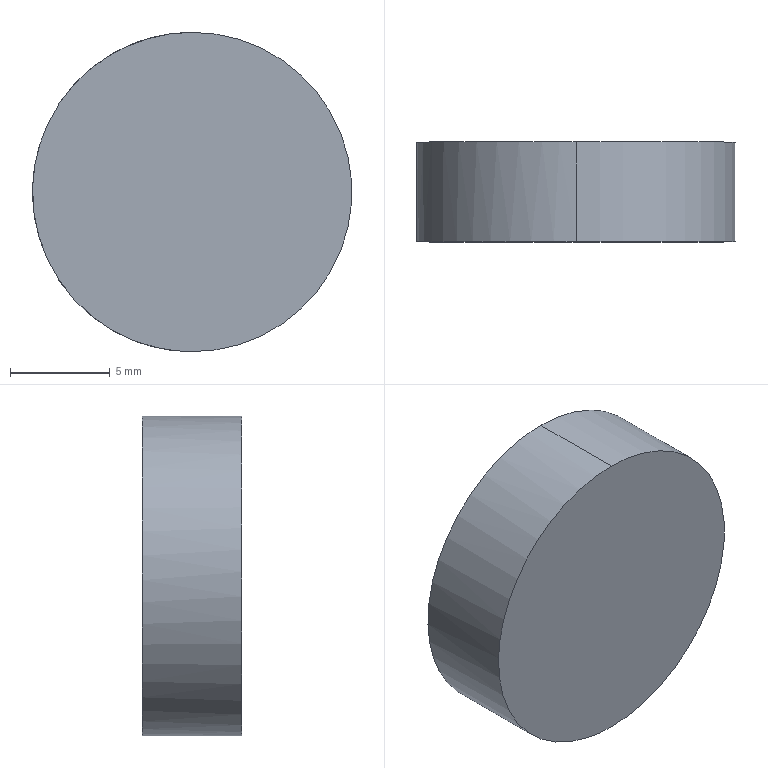Part | STEP file | Positioning_id1206_x_t | 1 solid | 4 faces | box 16 x 5 x 16 mm | volume 1005 mm3 | cylinder 2 | plane 2 | commonest cylinder face diameters 16 x2
STEP:
#1=CARTESIAN_POINT('',(0.,0.,0.));
#2=DIRECTION('',(0.,0.,1.));
#3=DIRECTION('',(1.,0.,0.));
#4=AXIS2_PLACEMENT_3D('',#1,#2,#3);
#5=CARTESIAN_POINT('',(-767.002,214.,185.532));
#6=VERTEX_POINT('',#5);
#7=CARTESIAN_POINT('',(-767.002,219.,185.532));
#8=VERTEX_POINT('',#7);
#9=CARTESIAN_POINT('',(-767.002,219.,185.532));
#10=DIRECTION('',(0.,1.,0.));
#11=VECTOR('',#10,1.);
#12=LINE('',#9,#11);
#13=CARTESIAN_POINT('',(-767.002,219.,193.532));
#14=DIRECTION('',(0.,1.,0.));
#15=DIRECTION('',(0.,0.,-1.));
#16=AXIS2_PLACEMENT_3D('',#13,#14,#15);
#17=CYLINDRICAL_SURFACE('',#16,8.);
#18=CARTESIAN_POINT('',(6.283,0.));
#19=DIRECTION('',(0.,1.));
#20=VECTOR('',#19,1.);
#21=LINE('',#18,#20);
#22=(GEOMETRIC_REPRESENTATION_CONTEXT(2)PARAMETRIC_REPRESENTATION_CONTEXT()REPRESENTATION_CONTEXT('',''));
#23=DEFINITIONAL_REPRESENTATION('',(#21),#22);
#24=PCURVE('',#17,#23);
#25=CARTESIAN_POINT('',(-767.002,219.,193.532));
#26=DIRECTION('',(0.,1.,0.));
#27=DIRECTION('',(0.,0.,-1.));
#28=AXIS2_PLACEMENT_3D('',#25,#26,#27);
#29=CYLINDRICAL_SURFACE('',#28,8.);
#30=CARTESIAN_POINT('',(0.,0.));
#31=DIRECTION('',(0.,1.));
#32=VECTOR('',#31,1.);
#33=LINE('',#30,#32);
#34=(GEOMETRIC_REPRESENTATION_CONTEXT(2)PARAMETRIC_REPRESENTATION_CONTEXT()REPRESENTATION_CONTEXT('',''));
#35=DEFINITIONAL_REPRESENTATION('',(#33),#34);
#36=PCURVE('',#29,#35);
#37=SURFACE_CURVE('',#12,(#24,#36),.PCURVE_S1.);
#38=EDGE_CURVE('',#6,#8,#37,.T.);
#39=ORIENTED_EDGE('',*,*,#38,.T.);
#40=CARTESIAN_POINT('',(-767.002,219.,201.532));
#41=VERTEX_POINT('',#40);
#42=CARTESIAN_POINT('',(-767.002,219.,193.532));
#43=DIRECTION('',(0.,1.,0.));
#44=DIRECTION('',(0.,0.,1.));
#45=AXIS2_PLACEMENT_3D('',#42,#43,#44);
#46=CIRCLE('',#45,8.);
#47=CARTESIAN_POINT('',(3.142,0.));
#48=DIRECTION('',(1.,0.));
#49=VECTOR('',#48,1.);
#50=LINE('',#47,#49);
#51=(GEOMETRIC_REPRESENTATION_CONTEXT(2)PARAMETRIC_REPRESENTATION_CONTEXT()REPRESENTATION_CONTEXT('',''));
#52=DEFINITIONAL_REPRESENTATION('',(#50),#51);
#53=PCURVE('',#17,#52);
#54=CARTESIAN_POINT('',(-767.002,219.,193.532));
#55=DIRECTION('',(0.,1.,0.));
#56=DIRECTION('',(0.,0.,1.));
#57=AXIS2_PLACEMENT_3D('',#54,#55,#56);
#58=PLANE('',#57);
#59=CARTESIAN_POINT('',(0.,0.));
#60=DIRECTION('',(1.,0.));
#61=AXIS2_PLACEMENT_2D('',#59,#60);
#62=CIRCLE('',#61,8.);
#63=(GEOMETRIC_REPRESENTATION_CONTEXT(2)PARAMETRIC_REPRESENTATION_CONTEXT()REPRESENTATION_CONTEXT('',''));
#64=DEFINITIONAL_REPRESENTATION('',(#62),#63);
#65=PCURVE('',#58,#64);
#66=SURFACE_CURVE('',#46,(#53,#65),.PCURVE_S1.);
#67=EDGE_CURVE('',#41,#8,#66,.T.);
#68=ORIENTED_EDGE('',*,*,#67,.F.);
#69=CARTESIAN_POINT('',(-767.002,214.,201.532));
#70=VERTEX_POINT('',#69);
#71=CARTESIAN_POINT('',(-767.002,219.,201.532));
#72=DIRECTION('',(0.,-1.,0.));
#73=VECTOR('',#72,1.);
#74=LINE('',#71,#73);
#75=CARTESIAN_POINT('',(3.142,0.));
#76=DIRECTION('',(0.,-1.));
#77=VECTOR('',#76,1.);
#78=LINE('',#75,#77);
#79=(GEOMETRIC_REPRESENTATION_CONTEXT(2)PARAMETRIC_REPRESENTATION_CONTEXT()REPRESENTATION_CONTEXT('',''));
#80=DEFINITIONAL_REPRESENTATION('',(#78),#79);
#81=PCURVE('',#17,#80);
#82=CARTESIAN_POINT('',(3.142,0.));
#83=DIRECTION('',(0.,-1.));
#84=VECTOR('',#83,1.);
#85=LINE('',#82,#84);
#86=(GEOMETRIC_REPRESENTATION_CONTEXT(2)PARAMETRIC_REPRESENTATION_CONTEXT()REPRESENTATION_CONTEXT('',''));
#87=DEFINITIONAL_REPRESENTATION('',(#85),#86);
#88=PCURVE('',#29,#87);
#89=SURFACE_CURVE('',#74,(#81,#88),.PCURVE_S1.);
#90=EDGE_CURVE('',#41,#70,#89,.T.);
#91=ORIENTED_EDGE('',*,*,#90,.T.);
#92=CARTESIAN_POINT('',(-767.002,214.,193.532));
#93=DIRECTION('',(0.,-1.,0.));
#94=DIRECTION('',(0.,0.,1.));
#95=AXIS2_PLACEMENT_3D('',#92,#93,#94);
#96=CIRCLE('',#95,8.);
#97=CARTESIAN_POINT('',(9.425,-5.));
#98=DIRECTION('',(-1.,0.));
#99=VECTOR('',#98,1.);
#100=LINE('',#97,#99);
#101=(GEOMETRIC_REPRESENTATION_CONTEXT(2)PARAMETRIC_REPRESENTATION_CONTEXT()REPRESENTATION_CONTEXT('',''));
#102=DEFINITIONAL_REPRESENTATION('',(#100),#101);
#103=PCURVE('',#17,#102);
#104=CARTESIAN_POINT('',(-767.002,214.,193.532));
#105=DIRECTION('',(0.,-1.,0.));
#106=DIRECTION('',(0.,0.,-1.));
#107=AXIS2_PLACEMENT_3D('',#104,#105,#106);
#108=PLANE('',#107);
#109=CARTESIAN_POINT('',(0.,0.));
#110=DIRECTION('',(-1.,0.));
#111=AXIS2_PLACEMENT_2D('',#109,#110);
#112=CIRCLE('',#111,8.);
#113=(GEOMETRIC_REPRESENTATION_CONTEXT(2)PARAMETRIC_REPRESENTATION_CONTEXT()REPRESENTATION_CONTEXT('',''));
#114=DEFINITIONAL_REPRESENTATION('',(#112),#113);
#115=PCURVE('',#108,#114);
#116=SURFACE_CURVE('',#96,(#103,#115),.PCURVE_S1.);
#117=EDGE_CURVE('',#6,#70,#116,.T.);
#118=ORIENTED_EDGE('',*,*,#117,.F.);
#119=EDGE_LOOP('',(#39,#68,#91,#118));
#120=FACE_BOUND('',#119,.T.);
#121=ADVANCED_FACE('',(#120),#17,.T.);
#122=ORIENTED_EDGE('',*,*,#67,.T.);
#123=CARTESIAN_POINT('',(-767.002,219.,185.532));
#124=CARTESIAN_POINT('',(-775.002,219.,185.532));
#125=CARTESIAN_POINT('',(-779.002,219.,193.532));
#126=CARTESIAN_POINT('',(-775.002,219.,201.532));
#127=CARTESIAN_POINT('',(-767.002,219.,201.532));
#128=(BOUNDED_CURVE()B_SPLINE_CURVE(4,(#123,#124,#125,#126,#127),.UNSPECIFIED.,.F.,.F.)B_SPLINE_CURVE_WITH_KNOTS((5,5),(0.,1.),.PIECEWISE_BEZIER_KNOTS.)CURVE()GEOMETRIC_REPRESENTATION_ITEM()RATIONAL_B_SPLINE_CURVE((1.,0.7071,0.6667,0.7071,1.))REPRESENTATION_ITEM(''));
#129=CARTESIAN_POINT('',(-8.,0.));
#130=CARTESIAN_POINT('',(-8.,-8.));
#131=CARTESIAN_POINT('',(0.,-12.));
#132=CARTESIAN_POINT('',(8.,-8.));
#133=CARTESIAN_POINT('',(8.,0.));
#134=(BOUNDED_CURVE()B_SPLINE_CURVE(4,(#129,#130,#131,#132,#133),.UNSPECIFIED.,.F.,.F.)B_SPLINE_CURVE_WITH_KNOTS((5,5),(0.,1.),.PIECEWISE_BEZIER_KNOTS.)CURVE()GEOMETRIC_REPRESENTATION_ITEM()RATIONAL_B_SPLINE_CURVE((1.,0.7071,0.6667,0.7071,1.))REPRESENTATION_ITEM(''));
#135=(GEOMETRIC_REPRESENTATION_CONTEXT(2)PARAMETRIC_REPRESENTATION_CONTEXT()REPRESENTATION_CONTEXT('',''));
#136=DEFINITIONAL_REPRESENTATION('',(#134),#135);
#137=PCURVE('',#58,#136);
#138=CARTESIAN_POINT('',(0.,0.));
#139=CARTESIAN_POINT('',(0.04285,0.));
#140=CARTESIAN_POINT('',(0.1297,0.));
#141=CARTESIAN_POINT('',(0.2633,0.));
#142=CARTESIAN_POINT('',(0.3999,0.));
#143=CARTESIAN_POINT('',(0.5394,0.));
#144=CARTESIAN_POINT('',(0.6816,0.));
#145=CARTESIAN_POINT('',(0.8261,0.));
#146=CARTESIAN_POINT('',(0.9725,0.));
#147=CARTESIAN_POINT('',(1.121,0.));
#148=CARTESIAN_POINT('',(1.27,0.));
#149=CARTESIAN_POINT('',(1.42,0.));
#150=CARTESIAN_POINT('',(1.571,0.));
#151=CARTESIAN_POINT('',(1.721,0.));
#152=CARTESIAN_POINT('',(1.872,0.));
#153=CARTESIAN_POINT('',(2.021,0.));
#154=CARTESIAN_POINT('',(2.169,0.));
#155=CARTESIAN_POINT('',(2.316,0.));
#156=CARTESIAN_POINT('',(2.46,0.));
#157=CARTESIAN_POINT('',(2.602,0.));
#158=CARTESIAN_POINT('',(2.742,0.));
#159=CARTESIAN_POINT('',(2.878,0.));
#160=CARTESIAN_POINT('',(3.012,0.));
#161=CARTESIAN_POINT('',(3.099,0.));
#162=CARTESIAN_POINT('',(3.142,0.));
#163=B_SPLINE_CURVE_WITH_KNOTS('',3,(#138,#139,#140,#141,#142,#143,#144,#145,#146,#147,#148,#149,#150,#151,#152,#153,#154,#155,#156,#157,#158,#159,#160,#161,#162),.UNSPECIFIED.,.F.,.F.,(4,1,1,1,1,1,1,1,1,1,1,1,1,1,1,1,1,1,1,1,1,1,4),(0.,0.04545,0.09091,0.1364,0.1818,0.2273,0.2727,0.3182,0.3636,0.4091,0.4545,0.5,0.5455,0.5909,0.6364,0.6818,0.7273,0.7727,0.8182,0.8636,0.9091,0.9545,1.),.QUASI_UNIFORM_KNOTS.);
#164=(GEOMETRIC_REPRESENTATION_CONTEXT(2)PARAMETRIC_REPRESENTATION_CONTEXT()REPRESENTATION_CONTEXT('',''));
#165=DEFINITIONAL_REPRESENTATION('',(#163),#164);
#166=PCURVE('',#29,#165);
#167=SURFACE_CURVE('',#128,(#137,#166),.PCURVE_S1.);
#168=EDGE_CURVE('',#8,#41,#167,.T.);
#169=ORIENTED_EDGE('',*,*,#168,.T.);
#170=EDGE_LOOP('',(#122,#169));
#171=FACE_BOUND('',#170,.T.);
#172=ADVANCED_FACE('',(#171),#58,.T.);
#173=CARTESIAN_POINT('',(-767.002,214.,201.532));
#174=CARTESIAN_POINT('',(-775.002,214.,201.532));
#175=CARTESIAN_POINT('',(-779.002,214.,193.532));
#176=CARTESIAN_POINT('',(-775.002,214.,185.532));
#177=CARTESIAN_POINT('',(-767.002,214.,185.532));
#178=(BOUNDED_CURVE()B_SPLINE_CURVE(4,(#173,#174,#175,#176,#177),.UNSPECIFIED.,.F.,.F.)B_SPLINE_CURVE_WITH_KNOTS((5,5),(0.,1.),.PIECEWISE_BEZIER_KNOTS.)CURVE()GEOMETRIC_REPRESENTATION_ITEM()RATIONAL_B_SPLINE_CURVE((1.,0.7071,0.6667,0.7071,1.))REPRESENTATION_ITEM(''));
#179=CARTESIAN_POINT('',(-8.,0.));
#180=CARTESIAN_POINT('',(-8.,-8.));
#181=CARTESIAN_POINT('',(0.,-12.));
#182=CARTESIAN_POINT('',(8.,-8.));
#183=CARTESIAN_POINT('',(8.,0.));
#184=(BOUNDED_CURVE()B_SPLINE_CURVE(4,(#179,#180,#181,#182,#183),.UNSPECIFIED.,.F.,.F.)B_SPLINE_CURVE_WITH_KNOTS((5,5),(0.,1.),.PIECEWISE_BEZIER_KNOTS.)CURVE()GEOMETRIC_REPRESENTATION_ITEM()RATIONAL_B_SPLINE_CURVE((1.,0.7071,0.6667,0.7071,1.))REPRESENTATION_ITEM(''));
#185=(GEOMETRIC_REPRESENTATION_CONTEXT(2)PARAMETRIC_REPRESENTATION_CONTEXT()REPRESENTATION_CONTEXT('',''));
#186=DEFINITIONAL_REPRESENTATION('',(#184),#185);
#187=PCURVE('',#108,#186);
#188=CARTESIAN_POINT('',(3.142,-5.));
#189=CARTESIAN_POINT('',(3.099,-5.));
#190=CARTESIAN_POINT('',(3.012,-5.));
#191=CARTESIAN_POINT('',(2.878,-5.));
#192=CARTESIAN_POINT('',(2.742,-5.));
#193=CARTESIAN_POINT('',(2.602,-5.));
#194=CARTESIAN_POINT('',(2.46,-5.));
#195=CARTESIAN_POINT('',(2.316,-5.));
#196=CARTESIAN_POINT('',(2.169,-5.));
#197=CARTESIAN_POINT('',(2.021,-5.));
#198=CARTESIAN_POINT('',(1.872,-5.));
#199=CARTESIAN_POINT('',(1.721,-5.));
#200=CARTESIAN_POINT('',(1.571,-5.));
#201=CARTESIAN_POINT('',(1.42,-5.));
#202=CARTESIAN_POINT('',(1.27,-5.));
#203=CARTESIAN_POINT('',(1.121,-5.));
#204=CARTESIAN_POINT('',(0.9725,-5.));
#205=CARTESIAN_POINT('',(0.8261,-5.));
#206=CARTESIAN_POINT('',(0.6816,-5.));
#207=CARTESIAN_POINT('',(0.5394,-5.));
#208=CARTESIAN_POINT('',(0.3999,-5.));
#209=CARTESIAN_POINT('',(0.2633,-5.));
#210=CARTESIAN_POINT('',(0.1297,-5.));
#211=CARTESIAN_POINT('',(0.04285,-5.));
#212=CARTESIAN_POINT('',(0.,-5.));
#213=B_SPLINE_CURVE_WITH_KNOTS('',3,(#188,#189,#190,#191,#192,#193,#194,#195,#196,#197,#198,#199,#200,#201,#202,#203,#204,#205,#206,#207,#208,#209,#210,#211,#212),.UNSPECIFIED.,.F.,.F.,(4,1,1,1,1,1,1,1,1,1,1,1,1,1,1,1,1,1,1,1,1,1,4),(0.,0.04545,0.09091,0.1364,0.1818,0.2273,0.2727,0.3182,0.3636,0.4091,0.4545,0.5,0.5455,0.5909,0.6364,0.6818,0.7273,0.7727,0.8182,0.8636,0.9091,0.9545,1.),.QUASI_UNIFORM_KNOTS.);
#214=(GEOMETRIC_REPRESENTATION_CONTEXT(2)PARAMETRIC_REPRESENTATION_CONTEXT()REPRESENTATION_CONTEXT('',''));
#215=DEFINITIONAL_REPRESENTATION('',(#213),#214);
#216=PCURVE('',#29,#215);
#217=SURFACE_CURVE('',#178,(#187,#216),.PCURVE_S1.);
#218=EDGE_CURVE('',#70,#6,#217,.T.);
#219=ORIENTED_EDGE('',*,*,#218,.T.);
#220=ORIENTED_EDGE('',*,*,#117,.T.);
#221=EDGE_LOOP('',(#219,#220));
#222=FACE_BOUND('',#221,.T.);
#223=ADVANCED_FACE('',(#222),#108,.T.);
#224=ORIENTED_EDGE('',*,*,#168,.F.);
#225=ORIENTED_EDGE('',*,*,#38,.F.);
#226=ORIENTED_EDGE('',*,*,#218,.F.);
#227=ORIENTED_EDGE('',*,*,#90,.F.);
#228=EDGE_LOOP('',(#224,#225,#226,#227));
#229=FACE_BOUND('',#228,.T.);
#230=ADVANCED_FACE('',(#229),#29,.T.);
#231=CLOSED_SHELL('',(#121,#172,#223,#230));
#232=MANIFOLD_SOLID_BREP('',#231);
#233=(LENGTH_UNIT()NAMED_UNIT(*)SI_UNIT(.MILLI.,.METRE.));
#234=UNCERTAINTY_MEASURE_WITH_UNIT(LENGTH_MEASURE(0.0000001),#233,'','');
#235=(NAMED_UNIT(*)PLANE_ANGLE_UNIT()SI_UNIT($,.RADIAN.));
#236=(NAMED_UNIT(*)SI_UNIT($,.STERADIAN.)SOLID_ANGLE_UNIT());
#237=(GEOMETRIC_REPRESENTATION_CONTEXT(3)GLOBAL_UNCERTAINTY_ASSIGNED_CONTEXT((#234))GLOBAL_UNIT_ASSIGNED_CONTEXT((#233,#235,#236))REPRESENTATION_CONTEXT('',''));
#238=ADVANCED_BREP_SHAPE_REPRESENTATION('',(#4,#232),#237);